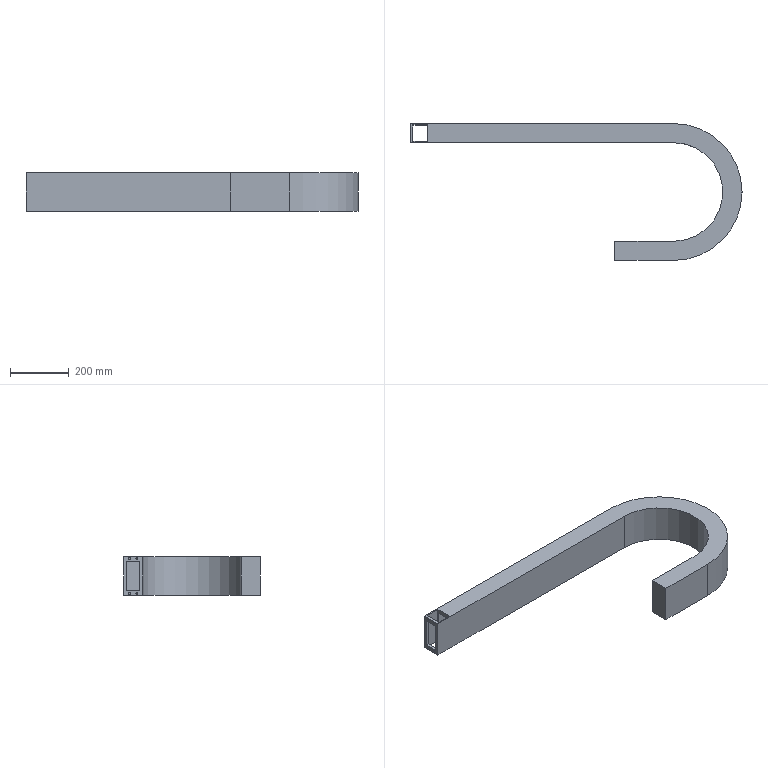Part | SolidWorks | features ICE 3, Extrusion 1 | 1 solid | 31 faces | box 1128 x 465 x 130 mm | volume 13528411 mm3 | plane 21 | cylinder 10 | commonest cylinder face diameters 6 x8 335 x1 465 x1
STEP:
#1=CARTESIAN_POINT('',(-5920.428,254.022,9.));
#2=VERTEX_POINT('',#1);
#3=CARTESIAN_POINT('',(-5920.428,254.022,3.));
#4=VERTEX_POINT('',#3);
#5=CARTESIAN_POINT('',(-5920.428,254.022,6.));
#6=DIRECTION('',(1.,0.,0.));
#7=DIRECTION('',(0.,0.,1.));
#8=AXIS2_PLACEMENT_3D('',#5,#6,#7);
#9=CIRCLE('',#8,3.);
#10=EDGE_CURVE('',#2,#4,#9,.T.);
#11=ORIENTED_EDGE('',*,*,#10,.T.);
#12=CARTESIAN_POINT('',(-5930.428,254.022,3.));
#13=VERTEX_POINT('',#12);
#14=CARTESIAN_POINT('',(-5910.428,254.022,3.));
#15=DIRECTION('',(-1.,0.,0.));
#16=VECTOR('',#15,1000.);
#17=LINE('',#14,#16);
#18=EDGE_CURVE('',#4,#13,#17,.T.);
#19=ORIENTED_EDGE('',*,*,#18,.T.);
#20=CARTESIAN_POINT('',(-5930.428,254.022,9.));
#21=VERTEX_POINT('',#20);
#22=CARTESIAN_POINT('',(-5930.428,254.022,6.));
#23=DIRECTION('',(-1.,0.,0.));
#24=DIRECTION('',(0.,0.,1.));
#25=AXIS2_PLACEMENT_3D('',#22,#23,#24);
#26=CIRCLE('',#25,3.);
#27=EDGE_CURVE('',#13,#21,#26,.T.);
#28=ORIENTED_EDGE('',*,*,#27,.T.);
#29=CARTESIAN_POINT('',(-5910.428,254.022,9.));
#30=DIRECTION('',(-1.,0.,0.));
#31=VECTOR('',#30,1000.);
#32=LINE('',#29,#31);
#33=EDGE_CURVE('',#2,#21,#32,.T.);
#34=ORIENTED_EDGE('',*,*,#33,.F.);
#35=EDGE_LOOP('',(#11,#19,#28,#34));
#36=FACE_OUTER_BOUND('',#35,.T.);
#37=CARTESIAN_POINT('',(-5910.428,254.022,6.));
#38=DIRECTION('',(-1.,0.,0.));
#39=DIRECTION('',(0.,0.,1.));
#40=AXIS2_PLACEMENT_3D('',#37,#38,#39);
#41=CYLINDRICAL_SURFACE('',#40,3.);
#42=ADVANCED_FACE('',(#36),#41,.F.);
#43=CARTESIAN_POINT('',(-5920.428,279.022,127.));
#44=VERTEX_POINT('',#43);
#45=CARTESIAN_POINT('',(-5920.428,279.022,121.));
#46=VERTEX_POINT('',#45);
#47=CARTESIAN_POINT('',(-5920.428,279.022,124.));
#48=DIRECTION('',(1.,0.,0.));
#49=DIRECTION('',(0.,0.,1.));
#50=AXIS2_PLACEMENT_3D('',#47,#48,#49);
#51=CIRCLE('',#50,3.);
#52=EDGE_CURVE('',#44,#46,#51,.T.);
#53=ORIENTED_EDGE('',*,*,#52,.T.);
#54=CARTESIAN_POINT('',(-5930.428,279.022,121.));
#55=VERTEX_POINT('',#54);
#56=CARTESIAN_POINT('',(-5910.428,279.022,121.));
#57=DIRECTION('',(-1.,0.,0.));
#58=VECTOR('',#57,1000.);
#59=LINE('',#56,#58);
#60=EDGE_CURVE('',#46,#55,#59,.T.);
#61=ORIENTED_EDGE('',*,*,#60,.T.);
#62=CARTESIAN_POINT('',(-5930.428,279.022,127.));
#63=VERTEX_POINT('',#62);
#64=CARTESIAN_POINT('',(-5930.428,279.022,124.));
#65=DIRECTION('',(-1.,0.,0.));
#66=DIRECTION('',(0.,0.,1.));
#67=AXIS2_PLACEMENT_3D('',#64,#65,#66);
#68=CIRCLE('',#67,3.);
#69=EDGE_CURVE('',#55,#63,#68,.T.);
#70=ORIENTED_EDGE('',*,*,#69,.T.);
#71=CARTESIAN_POINT('',(-5910.428,279.022,127.));
#72=DIRECTION('',(-1.,0.,0.));
#73=VECTOR('',#72,1000.);
#74=LINE('',#71,#73);
#75=EDGE_CURVE('',#44,#63,#74,.T.);
#76=ORIENTED_EDGE('',*,*,#75,.F.);
#77=EDGE_LOOP('',(#53,#61,#70,#76));
#78=FACE_OUTER_BOUND('',#77,.T.);
#79=CARTESIAN_POINT('',(-5910.428,279.022,124.));
#80=DIRECTION('',(-1.,0.,0.));
#81=DIRECTION('',(0.,0.,1.));
#82=AXIS2_PLACEMENT_3D('',#79,#80,#81);
#83=CYLINDRICAL_SURFACE('',#82,3.);
#84=ADVANCED_FACE('',(#78),#83,.F.);
#85=CARTESIAN_POINT('',(-5920.428,254.022,127.));
#86=VERTEX_POINT('',#85);
#87=CARTESIAN_POINT('',(-5920.428,254.022,121.));
#88=VERTEX_POINT('',#87);
#89=CARTESIAN_POINT('',(-5920.428,254.022,124.));
#90=DIRECTION('',(1.,0.,0.));
#91=DIRECTION('',(0.,0.,1.));
#92=AXIS2_PLACEMENT_3D('',#89,#90,#91);
#93=CIRCLE('',#92,3.);
#94=EDGE_CURVE('',#86,#88,#93,.T.);
#95=ORIENTED_EDGE('',*,*,#94,.T.);
#96=CARTESIAN_POINT('',(-5930.428,254.022,121.));
#97=VERTEX_POINT('',#96);
#98=CARTESIAN_POINT('',(-5910.428,254.022,121.));
#99=DIRECTION('',(-1.,0.,0.));
#100=VECTOR('',#99,1000.);
#101=LINE('',#98,#100);
#102=EDGE_CURVE('',#88,#97,#101,.T.);
#103=ORIENTED_EDGE('',*,*,#102,.T.);
#104=CARTESIAN_POINT('',(-5930.428,254.022,127.));
#105=VERTEX_POINT('',#104);
#106=CARTESIAN_POINT('',(-5930.428,254.022,124.));
#107=DIRECTION('',(-1.,0.,0.));
#108=DIRECTION('',(0.,0.,1.));
#109=AXIS2_PLACEMENT_3D('',#106,#107,#108);
#110=CIRCLE('',#109,3.);
#111=EDGE_CURVE('',#97,#105,#110,.T.);
#112=ORIENTED_EDGE('',*,*,#111,.T.);
#113=CARTESIAN_POINT('',(-5910.428,254.022,127.));
#114=DIRECTION('',(-1.,0.,0.));
#115=VECTOR('',#114,1000.);
#116=LINE('',#113,#115);
#117=EDGE_CURVE('',#86,#105,#116,.T.);
#118=ORIENTED_EDGE('',*,*,#117,.F.);
#119=EDGE_LOOP('',(#95,#103,#112,#118));
#120=FACE_OUTER_BOUND('',#119,.T.);
#121=CARTESIAN_POINT('',(-5910.428,254.022,124.));
#122=DIRECTION('',(-1.,0.,0.));
#123=DIRECTION('',(0.,0.,1.));
#124=AXIS2_PLACEMENT_3D('',#121,#122,#123);
#125=CYLINDRICAL_SURFACE('',#124,3.);
#126=ADVANCED_FACE('',(#120),#125,.F.);
#127=CARTESIAN_POINT('',(-5920.428,279.022,9.));
#128=VERTEX_POINT('',#127);
#129=CARTESIAN_POINT('',(-5920.428,279.022,3.));
#130=VERTEX_POINT('',#129);
#131=CARTESIAN_POINT('',(-5920.428,279.022,6.));
#132=DIRECTION('',(1.,0.,0.));
#133=DIRECTION('',(0.,0.,1.));
#134=AXIS2_PLACEMENT_3D('',#131,#132,#133);
#135=CIRCLE('',#134,3.);
#136=EDGE_CURVE('',#128,#130,#135,.T.);
#137=ORIENTED_EDGE('',*,*,#136,.T.);
#138=CARTESIAN_POINT('',(-5930.428,279.022,3.));
#139=VERTEX_POINT('',#138);
#140=CARTESIAN_POINT('',(-5910.428,279.022,3.));
#141=DIRECTION('',(-1.,0.,0.));
#142=VECTOR('',#141,1000.);
#143=LINE('',#140,#142);
#144=EDGE_CURVE('',#130,#139,#143,.T.);
#145=ORIENTED_EDGE('',*,*,#144,.T.);
#146=CARTESIAN_POINT('',(-5930.428,279.022,9.));
#147=VERTEX_POINT('',#146);
#148=CARTESIAN_POINT('',(-5930.428,279.022,6.));
#149=DIRECTION('',(-1.,0.,0.));
#150=DIRECTION('',(0.,0.,1.));
#151=AXIS2_PLACEMENT_3D('',#148,#149,#150);
#152=CIRCLE('',#151,3.);
#153=EDGE_CURVE('',#139,#147,#152,.T.);
#154=ORIENTED_EDGE('',*,*,#153,.T.);
#155=CARTESIAN_POINT('',(-5910.428,279.022,9.));
#156=DIRECTION('',(-1.,0.,0.));
#157=VECTOR('',#156,1000.);
#158=LINE('',#155,#157);
#159=EDGE_CURVE('',#128,#147,#158,.T.);
#160=ORIENTED_EDGE('',*,*,#159,.F.);
#161=EDGE_LOOP('',(#137,#145,#154,#160));
#162=FACE_OUTER_BOUND('',#161,.T.);
#163=CARTESIAN_POINT('',(-5910.428,279.022,6.));
#164=DIRECTION('',(-1.,0.,0.));
#165=DIRECTION('',(0.,0.,1.));
#166=AXIS2_PLACEMENT_3D('',#163,#164,#165);
#167=CYLINDRICAL_SURFACE('',#166,3.);
#168=ADVANCED_FACE('',(#162),#167,.F.);
#169=CARTESIAN_POINT('',(-5035.428,-165.978,0.));
#170=VERTEX_POINT('',#169);
#171=CARTESIAN_POINT('',(-5035.428,299.022,0.));
#172=VERTEX_POINT('',#171);
#173=CARTESIAN_POINT('',(-5035.428,66.522,0.));
#174=DIRECTION('',(0.,0.,1.));
#175=DIRECTION('',(1.,0.,0.));
#176=AXIS2_PLACEMENT_3D('',#173,#174,#175);
#177=CIRCLE('',#176,232.5);
#178=EDGE_CURVE('',#170,#172,#177,.T.);
#179=ORIENTED_EDGE('',*,*,#178,.T.);
#180=CARTESIAN_POINT('',(-5035.428,299.022,130.));
#181=VERTEX_POINT('',#180);
#182=CARTESIAN_POINT('',(-5035.428,299.022,130.));
#183=DIRECTION('',(0.,0.,-1.));
#184=VECTOR('',#183,1000.);
#185=LINE('',#182,#184);
#186=EDGE_CURVE('',#181,#172,#185,.T.);
#187=ORIENTED_EDGE('',*,*,#186,.F.);
#188=CARTESIAN_POINT('',(-5035.428,-165.978,130.));
#189=VERTEX_POINT('',#188);
#190=CARTESIAN_POINT('',(-5035.428,66.522,130.));
#191=DIRECTION('',(0.,0.,1.));
#192=DIRECTION('',(1.,0.,0.));
#193=AXIS2_PLACEMENT_3D('',#190,#191,#192);
#194=CIRCLE('',#193,232.5);
#195=EDGE_CURVE('',#189,#181,#194,.T.);
#196=ORIENTED_EDGE('',*,*,#195,.F.);
#197=CARTESIAN_POINT('',(-5035.428,-165.978,130.));
#198=DIRECTION('',(0.,0.,-1.));
#199=VECTOR('',#198,1000.);
#200=LINE('',#197,#199);
#201=EDGE_CURVE('',#189,#170,#200,.T.);
#202=ORIENTED_EDGE('',*,*,#201,.T.);
#203=EDGE_LOOP('',(#179,#187,#196,#202));
#204=FACE_OUTER_BOUND('',#203,.T.);
#205=CARTESIAN_POINT('',(-5035.428,66.522,130.));
#206=DIRECTION('',(0.,0.,-1.));
#207=DIRECTION('',(-1.,0.,0.));
#208=AXIS2_PLACEMENT_3D('',#205,#206,#207);
#209=CYLINDRICAL_SURFACE('',#208,232.5);
#210=ADVANCED_FACE('',(#204),#209,.T.);
#211=CARTESIAN_POINT('',(-5930.428,299.022,0.));
#212=VERTEX_POINT('',#211);
#213=CARTESIAN_POINT('',(-5035.428,299.022,0.));
#214=DIRECTION('',(-1.,0.,0.));
#215=VECTOR('',#214,1000.);
#216=LINE('',#213,#215);
#217=EDGE_CURVE('',#172,#212,#216,.T.);
#218=ORIENTED_EDGE('',*,*,#217,.T.);
#219=CARTESIAN_POINT('',(-5930.428,299.022,130.));
#220=VERTEX_POINT('',#219);
#221=CARTESIAN_POINT('',(-5930.428,299.022,130.));
#222=DIRECTION('',(0.,0.,-1.));
#223=VECTOR('',#222,1000.);
#224=LINE('',#221,#223);
#225=EDGE_CURVE('',#220,#212,#224,.T.);
#226=ORIENTED_EDGE('',*,*,#225,.F.);
#227=CARTESIAN_POINT('',(-5035.428,299.022,130.));
#228=DIRECTION('',(-1.,0.,0.));
#229=VECTOR('',#228,1000.);
#230=LINE('',#227,#229);
#231=EDGE_CURVE('',#181,#220,#230,.T.);
#232=ORIENTED_EDGE('',*,*,#231,.F.);
#233=ORIENTED_EDGE('',*,*,#186,.T.);
#234=EDGE_LOOP('',(#218,#226,#232,#233));
#235=FACE_OUTER_BOUND('',#234,.T.);
#236=CARTESIAN_POINT('',(-5035.428,299.022,130.));
#237=DIRECTION('',(0.,-1.,0.));
#238=DIRECTION('',(1.,0.,0.));
#239=AXIS2_PLACEMENT_3D('',#236,#237,#238);
#240=PLANE('',#239);
#241=ADVANCED_FACE('',(#235),#240,.F.);
#242=CARTESIAN_POINT('',(-5930.428,244.022,15.));
#243=VERTEX_POINT('',#242);
#244=CARTESIAN_POINT('',(-5930.428,244.022,115.));
#245=VERTEX_POINT('',#244);
#246=CARTESIAN_POINT('',(-5930.428,244.022,15.));
#247=DIRECTION('',(0.,0.,1.));
#248=VECTOR('',#247,1000.);
#249=LINE('',#246,#248);
#250=EDGE_CURVE('',#243,#245,#249,.T.);
#251=ORIENTED_EDGE('',*,*,#250,.F.);
#252=CARTESIAN_POINT('',(-5930.428,289.022,15.));
#253=VERTEX_POINT('',#252);
#254=CARTESIAN_POINT('',(-5930.428,289.022,15.));
#255=DIRECTION('',(0.,-1.,0.));
#256=VECTOR('',#255,1000.);
#257=LINE('',#254,#256);
#258=EDGE_CURVE('',#253,#243,#257,.T.);
#259=ORIENTED_EDGE('',*,*,#258,.F.);
#260=CARTESIAN_POINT('',(-5930.428,289.022,115.));
#261=VERTEX_POINT('',#260);
#262=CARTESIAN_POINT('',(-5930.428,289.022,15.));
#263=DIRECTION('',(0.,0.,-1.));
#264=VECTOR('',#263,1000.);
#265=LINE('',#262,#264);
#266=EDGE_CURVE('',#261,#253,#265,.T.);
#267=ORIENTED_EDGE('',*,*,#266,.F.);
#268=CARTESIAN_POINT('',(-5930.428,289.022,115.));
#269=DIRECTION('',(0.,1.,0.));
#270=VECTOR('',#269,1000.);
#271=LINE('',#268,#270);
#272=EDGE_CURVE('',#245,#261,#271,.T.);
#273=ORIENTED_EDGE('',*,*,#272,.F.);
#274=EDGE_LOOP('',(#251,#259,#267,#273));
#275=FACE_BOUND('',#274,.T.);
#276=CARTESIAN_POINT('',(-5930.428,254.022,6.));
#277=DIRECTION('',(-1.,0.,0.));
#278=DIRECTION('',(0.,0.,1.));
#279=AXIS2_PLACEMENT_3D('',#276,#277,#278);
#280=CIRCLE('',#279,3.);
#281=EDGE_CURVE('',#21,#13,#280,.T.);
#282=ORIENTED_EDGE('',*,*,#281,.F.);
#283=ORIENTED_EDGE('',*,*,#27,.F.);
#284=EDGE_LOOP('',(#282,#283));
#285=FACE_BOUND('',#284,.T.);
#286=CARTESIAN_POINT('',(-5930.428,279.022,124.));
#287=DIRECTION('',(-1.,0.,0.));
#288=DIRECTION('',(0.,0.,1.));
#289=AXIS2_PLACEMENT_3D('',#286,#287,#288);
#290=CIRCLE('',#289,3.);
#291=EDGE_CURVE('',#63,#55,#290,.T.);
#292=ORIENTED_EDGE('',*,*,#291,.F.);
#293=ORIENTED_EDGE('',*,*,#69,.F.);
#294=EDGE_LOOP('',(#292,#293));
#295=FACE_BOUND('',#294,.T.);
#296=CARTESIAN_POINT('',(-5930.428,254.022,124.));
#297=DIRECTION('',(-1.,0.,0.));
#298=DIRECTION('',(0.,0.,1.));
#299=AXIS2_PLACEMENT_3D('',#296,#297,#298);
#300=CIRCLE('',#299,3.);
#301=EDGE_CURVE('',#105,#97,#300,.T.);
#302=ORIENTED_EDGE('',*,*,#301,.F.);
#303=ORIENTED_EDGE('',*,*,#111,.F.);
#304=EDGE_LOOP('',(#302,#303));
#305=FACE_BOUND('',#304,.T.);
#306=CARTESIAN_POINT('',(-5930.428,279.022,6.));
#307=DIRECTION('',(-1.,0.,0.));
#308=DIRECTION('',(0.,0.,1.));
#309=AXIS2_PLACEMENT_3D('',#306,#307,#308);
#310=CIRCLE('',#309,3.);
#311=EDGE_CURVE('',#147,#139,#310,.T.);
#312=ORIENTED_EDGE('',*,*,#311,.F.);
#313=ORIENTED_EDGE('',*,*,#153,.F.);
#314=EDGE_LOOP('',(#312,#313));
#315=FACE_BOUND('',#314,.T.);
#316=CARTESIAN_POINT('',(-5930.428,234.022,0.));
#317=VERTEX_POINT('',#316);
#318=CARTESIAN_POINT('',(-5930.428,299.022,0.));
#319=DIRECTION('',(0.,-1.,0.));
#320=VECTOR('',#319,1000.);
#321=LINE('',#318,#320);
#322=EDGE_CURVE('',#212,#317,#321,.T.);
#323=ORIENTED_EDGE('',*,*,#322,.T.);
#324=CARTESIAN_POINT('',(-5930.428,234.022,130.));
#325=VERTEX_POINT('',#324);
#326=CARTESIAN_POINT('',(-5930.428,234.022,130.));
#327=DIRECTION('',(0.,0.,-1.));
#328=VECTOR('',#327,1000.);
#329=LINE('',#326,#328);
#330=EDGE_CURVE('',#325,#317,#329,.T.);
#331=ORIENTED_EDGE('',*,*,#330,.F.);
#332=CARTESIAN_POINT('',(-5930.428,299.022,130.));
#333=DIRECTION('',(0.,-1.,0.));
#334=VECTOR('',#333,1000.);
#335=LINE('',#332,#334);
#336=EDGE_CURVE('',#220,#325,#335,.T.);
#337=ORIENTED_EDGE('',*,*,#336,.F.);
#338=ORIENTED_EDGE('',*,*,#225,.T.);
#339=EDGE_LOOP('',(#323,#331,#337,#338));
#340=FACE_OUTER_BOUND('',#339,.T.);
#341=CARTESIAN_POINT('',(-5930.428,299.022,130.));
#342=DIRECTION('',(1.,0.,0.));
#343=DIRECTION('',(0.,0.,-1.));
#344=AXIS2_PLACEMENT_3D('',#341,#342,#343);
#345=PLANE('',#344);
#346=ADVANCED_FACE('',(#275,#285,#295,#305,#315,#340),#345,.F.);
#347=CARTESIAN_POINT('',(-5035.428,234.022,0.));
#348=VERTEX_POINT('',#347);
#349=CARTESIAN_POINT('',(-5035.428,234.022,0.));
#350=DIRECTION('',(1.,0.,0.));
#351=VECTOR('',#350,1000.);
#352=LINE('',#349,#351);
#353=EDGE_CURVE('',#317,#348,#352,.T.);
#354=ORIENTED_EDGE('',*,*,#353,.T.);
#355=CARTESIAN_POINT('',(-5035.428,234.022,130.));
#356=VERTEX_POINT('',#355);
#357=CARTESIAN_POINT('',(-5035.428,234.022,130.));
#358=DIRECTION('',(0.,0.,-1.));
#359=VECTOR('',#358,1000.);
#360=LINE('',#357,#359);
#361=EDGE_CURVE('',#356,#348,#360,.T.);
#362=ORIENTED_EDGE('',*,*,#361,.F.);
#363=CARTESIAN_POINT('',(-5035.428,234.022,130.));
#364=DIRECTION('',(1.,0.,0.));
#365=VECTOR('',#364,1000.);
#366=LINE('',#363,#365);
#367=EDGE_CURVE('',#325,#356,#366,.T.);
#368=ORIENTED_EDGE('',*,*,#367,.F.);
#369=ORIENTED_EDGE('',*,*,#330,.T.);
#370=EDGE_LOOP('',(#354,#362,#368,#369));
#371=FACE_OUTER_BOUND('',#370,.T.);
#372=CARTESIAN_POINT('',(-5035.428,234.022,130.));
#373=DIRECTION('',(0.,1.,0.));
#374=DIRECTION('',(-1.,0.,0.));
#375=AXIS2_PLACEMENT_3D('',#372,#373,#374);
#376=PLANE('',#375);
#377=ADVANCED_FACE('',(#371),#376,.F.);
#378=CARTESIAN_POINT('',(-5035.428,-100.978,0.));
#379=VERTEX_POINT('',#378);
#380=CARTESIAN_POINT('',(-5035.428,66.522,0.));
#381=DIRECTION('',(0.,0.,-1.));
#382=DIRECTION('',(1.,0.,0.));
#383=AXIS2_PLACEMENT_3D('',#380,#381,#382);
#384=CIRCLE('',#383,167.5);
#385=EDGE_CURVE('',#348,#379,#384,.T.);
#386=ORIENTED_EDGE('',*,*,#385,.T.);
#387=CARTESIAN_POINT('',(-5035.428,-100.978,130.));
#388=VERTEX_POINT('',#387);
#389=CARTESIAN_POINT('',(-5035.428,-100.978,130.));
#390=DIRECTION('',(0.,0.,-1.));
#391=VECTOR('',#390,1000.);
#392=LINE('',#389,#391);
#393=EDGE_CURVE('',#388,#379,#392,.T.);
#394=ORIENTED_EDGE('',*,*,#393,.F.);
#395=CARTESIAN_POINT('',(-5035.428,66.522,130.));
#396=DIRECTION('',(0.,0.,-1.));
#397=DIRECTION('',(1.,0.,0.));
#398=AXIS2_PLACEMENT_3D('',#395,#396,#397);
#399=CIRCLE('',#398,167.5);
#400=EDGE_CURVE('',#356,#388,#399,.T.);
#401=ORIENTED_EDGE('',*,*,#400,.F.);
#402=ORIENTED_EDGE('',*,*,#361,.T.);
#403=EDGE_LOOP('',(#386,#394,#401,#402));
#404=FACE_OUTER_BOUND('',#403,.T.);
#405=CARTESIAN_POINT('',(-5035.428,66.522,130.));
#406=DIRECTION('',(0.,0.,-1.));
#407=DIRECTION('',(-1.,0.,0.));
#408=AXIS2_PLACEMENT_3D('',#405,#406,#407);
#409=CYLINDRICAL_SURFACE('',#408,167.5);
#410=ADVANCED_FACE('',(#404),#409,.F.);
#411=CARTESIAN_POINT('',(-5235.428,-100.978,0.));
#412=VERTEX_POINT('',#411);
#413=CARTESIAN_POINT('',(-5035.428,-100.978,0.));
#414=DIRECTION('',(-1.,0.,0.));
#415=VECTOR('',#414,1000.);
#416=LINE('',#413,#415);
#417=EDGE_CURVE('',#379,#412,#416,.T.);
#418=ORIENTED_EDGE('',*,*,#417,.T.);
#419=CARTESIAN_POINT('',(-5235.428,-100.978,130.));
#420=VERTEX_POINT('',#419);
#421=CARTESIAN_POINT('',(-5235.428,-100.978,130.));
#422=DIRECTION('',(0.,0.,-1.));
#423=VECTOR('',#422,1000.);
#424=LINE('',#421,#423);
#425=EDGE_CURVE('',#420,#412,#424,.T.);
#426=ORIENTED_EDGE('',*,*,#425,.F.);
#427=CARTESIAN_POINT('',(-5035.428,-100.978,130.));
#428=DIRECTION('',(-1.,0.,0.));
#429=VECTOR('',#428,1000.);
#430=LINE('',#427,#429);
#431=EDGE_CURVE('',#388,#420,#430,.T.);
#432=ORIENTED_EDGE('',*,*,#431,.F.);
#433=ORIENTED_EDGE('',*,*,#393,.T.);
#434=EDGE_LOOP('',(#418,#426,#432,#433));
#435=FACE_OUTER_BOUND('',#434,.T.);
#436=CARTESIAN_POINT('',(-5035.428,-100.978,130.));
#437=DIRECTION('',(0.,-1.,0.));
#438=DIRECTION('',(1.,0.,0.));
#439=AXIS2_PLACEMENT_3D('',#436,#437,#438);
#440=PLANE('',#439);
#441=ADVANCED_FACE('',(#435),#440,.F.);
#442=CARTESIAN_POINT('',(-5235.428,-165.978,0.));
#443=VERTEX_POINT('',#442);
#444=CARTESIAN_POINT('',(-5235.428,-165.978,0.));
#445=DIRECTION('',(0.,-1.,0.));
#446=VECTOR('',#445,1000.);
#447=LINE('',#444,#446);
#448=EDGE_CURVE('',#412,#443,#447,.T.);
#449=ORIENTED_EDGE('',*,*,#448,.T.);
#450=CARTESIAN_POINT('',(-5235.428,-165.978,130.));
#451=VERTEX_POINT('',#450);
#452=CARTESIAN_POINT('',(-5235.428,-165.978,130.));
#453=DIRECTION('',(0.,0.,-1.));
#454=VECTOR('',#453,1000.);
#455=LINE('',#452,#454);
#456=EDGE_CURVE('',#451,#443,#455,.T.);
#457=ORIENTED_EDGE('',*,*,#456,.F.);
#458=CARTESIAN_POINT('',(-5235.428,-165.978,130.));
#459=DIRECTION('',(0.,-1.,0.));
#460=VECTOR('',#459,1000.);
#461=LINE('',#458,#460);
#462=EDGE_CURVE('',#420,#451,#461,.T.);
#463=ORIENTED_EDGE('',*,*,#462,.F.);
#464=ORIENTED_EDGE('',*,*,#425,.T.);
#465=EDGE_LOOP('',(#449,#457,#463,#464));
#466=FACE_OUTER_BOUND('',#465,.T.);
#467=CARTESIAN_POINT('',(-5235.428,-165.978,130.));
#468=DIRECTION('',(1.,0.,0.));
#469=DIRECTION('',(0.,0.,-1.));
#470=AXIS2_PLACEMENT_3D('',#467,#468,#469);
#471=PLANE('',#470);
#472=ADVANCED_FACE('',(#466),#471,.F.);
#473=CARTESIAN_POINT('',(-5035.428,-165.978,0.));
#474=DIRECTION('',(1.,0.,0.));
#475=VECTOR('',#474,1000.);
#476=LINE('',#473,#475);
#477=EDGE_CURVE('',#443,#170,#476,.T.);
#478=ORIENTED_EDGE('',*,*,#477,.T.);
#479=ORIENTED_EDGE('',*,*,#201,.F.);
#480=CARTESIAN_POINT('',(-5035.428,-165.978,130.));
#481=DIRECTION('',(1.,0.,0.));
#482=VECTOR('',#481,1000.);
#483=LINE('',#480,#482);
#484=EDGE_CURVE('',#451,#189,#483,.T.);
#485=ORIENTED_EDGE('',*,*,#484,.F.);
#486=ORIENTED_EDGE('',*,*,#456,.T.);
#487=EDGE_LOOP('',(#478,#479,#485,#486));
#488=FACE_OUTER_BOUND('',#487,.T.);
#489=CARTESIAN_POINT('',(-5035.428,-165.978,130.));
#490=DIRECTION('',(0.,1.,0.));
#491=DIRECTION('',(-1.,0.,0.));
#492=AXIS2_PLACEMENT_3D('',#489,#490,#491);
#493=PLANE('',#492);
#494=ADVANCED_FACE('',(#488),#493,.F.);
#495=CARTESIAN_POINT('',(-5920.428,294.022,130.));
#496=VERTEX_POINT('',#495);
#497=CARTESIAN_POINT('',(-5920.428,239.022,130.));
#498=VERTEX_POINT('',#497);
#499=CARTESIAN_POINT('',(-5920.428,294.022,130.));
#500=DIRECTION('',(0.,-1.,0.));
#501=VECTOR('',#500,1000.);
#502=LINE('',#499,#501);
#503=EDGE_CURVE('',#496,#498,#502,.T.);
#504=ORIENTED_EDGE('',*,*,#503,.F.);
#505=CARTESIAN_POINT('',(-5870.428,294.022,130.));
#506=VERTEX_POINT('',#505);
#507=CARTESIAN_POINT('',(-5920.428,294.022,130.));
#508=DIRECTION('',(-1.,0.,0.));
#509=VECTOR('',#508,1000.);
#510=LINE('',#507,#509);
#511=EDGE_CURVE('',#506,#496,#510,.T.);
#512=ORIENTED_EDGE('',*,*,#511,.F.);
#513=CARTESIAN_POINT('',(-5870.428,239.022,130.));
#514=VERTEX_POINT('',#513);
#515=CARTESIAN_POINT('',(-5870.428,294.022,130.));
#516=DIRECTION('',(0.,1.,0.));
#517=VECTOR('',#516,1000.);
#518=LINE('',#515,#517);
#519=EDGE_CURVE('',#514,#506,#518,.T.);
#520=ORIENTED_EDGE('',*,*,#519,.F.);
#521=CARTESIAN_POINT('',(-5920.428,239.022,130.));
#522=DIRECTION('',(1.,0.,0.));
#523=VECTOR('',#522,1000.);
#524=LINE('',#521,#523);
#525=EDGE_CURVE('',#498,#514,#524,.T.);
#526=ORIENTED_EDGE('',*,*,#525,.F.);
#527=EDGE_LOOP('',(#504,#512,#520,#526));
#528=FACE_BOUND('',#527,.T.);
#529=ORIENTED_EDGE('',*,*,#195,.T.);
#530=ORIENTED_EDGE('',*,*,#231,.T.);
#531=ORIENTED_EDGE('',*,*,#336,.T.);
#532=ORIENTED_EDGE('',*,*,#367,.T.);
#533=ORIENTED_EDGE('',*,*,#400,.T.);
#534=ORIENTED_EDGE('',*,*,#431,.T.);
#535=ORIENTED_EDGE('',*,*,#462,.T.);
#536=ORIENTED_EDGE('',*,*,#484,.T.);
#537=EDGE_LOOP('',(#529,#530,#531,#532,#533,#534,#535,#536));
#538=FACE_OUTER_BOUND('',#537,.T.);
#539=CARTESIAN_POINT('',(-5035.428,66.522,130.));
#540=DIRECTION('',(0.,0.,1.));
#541=DIRECTION('',(1.,0.,0.));
#542=AXIS2_PLACEMENT_3D('',#539,#540,#541);
#543=PLANE('',#542);
#544=ADVANCED_FACE('',(#528,#538),#543,.T.);
#545=CARTESIAN_POINT('',(-5870.428,294.022,0.));
#546=VERTEX_POINT('',#545);
#547=CARTESIAN_POINT('',(-5920.428,294.022,0.));
#548=VERTEX_POINT('',#547);
#549=CARTESIAN_POINT('',(-5035.428,294.022,0.));
#550=DIRECTION('',(-1.,0.,0.));
#551=VECTOR('',#550,1000.);
#552=LINE('',#549,#551);
#553=EDGE_CURVE('',#546,#548,#552,.T.);
#554=ORIENTED_EDGE('',*,*,#553,.T.);
#555=CARTESIAN_POINT('',(-5920.428,239.022,0.));
#556=VERTEX_POINT('',#555);
#557=CARTESIAN_POINT('',(-5920.428,66.522,0.));
#558=DIRECTION('',(0.,-1.,0.));
#559=VECTOR('',#558,1000.);
#560=LINE('',#557,#559);
#561=EDGE_CURVE('',#548,#556,#560,.T.);
#562=ORIENTED_EDGE('',*,*,#561,.T.);
#563=CARTESIAN_POINT('',(-5870.428,239.022,0.));
#564=VERTEX_POINT('',#563);
#565=CARTESIAN_POINT('',(-5035.428,239.022,0.));
#566=DIRECTION('',(1.,0.,0.));
#567=VECTOR('',#566,1000.);
#568=LINE('',#565,#567);
#569=EDGE_CURVE('',#556,#564,#568,.T.);
#570=ORIENTED_EDGE('',*,*,#569,.T.);
#571=CARTESIAN_POINT('',(-5870.428,66.522,0.));
#572=DIRECTION('',(0.,1.,0.));
#573=VECTOR('',#572,1000.);
#574=LINE('',#571,#573);
#575=EDGE_CURVE('',#564,#546,#574,.T.);
#576=ORIENTED_EDGE('',*,*,#575,.T.);
#577=EDGE_LOOP('',(#554,#562,#570,#576));
#578=FACE_BOUND('',#577,.T.);
#579=ORIENTED_EDGE('',*,*,#178,.F.);
#580=ORIENTED_EDGE('',*,*,#477,.F.);
#581=ORIENTED_EDGE('',*,*,#448,.F.);
#582=ORIENTED_EDGE('',*,*,#417,.F.);
#583=ORIENTED_EDGE('',*,*,#385,.F.);
#584=ORIENTED_EDGE('',*,*,#353,.F.);
#585=ORIENTED_EDGE('',*,*,#322,.F.);
#586=ORIENTED_EDGE('',*,*,#217,.F.);
#587=EDGE_LOOP('',(#579,#580,#581,#582,#583,#584,#585,#586));
#588=FACE_OUTER_BOUND('',#587,.T.);
#589=CARTESIAN_POINT('',(-5035.428,66.522,0.));
#590=DIRECTION('',(0.,0.,1.));
#591=DIRECTION('',(1.,0.,0.));
#592=AXIS2_PLACEMENT_3D('',#589,#590,#591);
#593=PLANE('',#592);
#594=ADVANCED_FACE('',(#578,#588),#593,.F.);
#595=ORIENTED_EDGE('',*,*,#144,.F.);
#596=CARTESIAN_POINT('',(-5920.428,279.022,6.));
#597=DIRECTION('',(1.,0.,0.));
#598=DIRECTION('',(0.,0.,1.));
#599=AXIS2_PLACEMENT_3D('',#596,#597,#598);
#600=CIRCLE('',#599,3.);
#601=EDGE_CURVE('',#130,#128,#600,.T.);
#602=ORIENTED_EDGE('',*,*,#601,.T.);
#603=ORIENTED_EDGE('',*,*,#159,.T.);
#604=ORIENTED_EDGE('',*,*,#311,.T.);
#605=EDGE_LOOP('',(#595,#602,#603,#604));
#606=FACE_OUTER_BOUND('',#605,.T.);
#607=CARTESIAN_POINT('',(-5910.428,279.022,6.));
#608=DIRECTION('',(-1.,0.,0.));
#609=DIRECTION('',(0.,0.,1.));
#610=AXIS2_PLACEMENT_3D('',#607,#608,#609);
#611=CYLINDRICAL_SURFACE('',#610,3.);
#612=ADVANCED_FACE('',(#606),#611,.F.);
#613=ORIENTED_EDGE('',*,*,#102,.F.);
#614=CARTESIAN_POINT('',(-5920.428,254.022,124.));
#615=DIRECTION('',(1.,0.,0.));
#616=DIRECTION('',(0.,0.,1.));
#617=AXIS2_PLACEMENT_3D('',#614,#615,#616);
#618=CIRCLE('',#617,3.);
#619=EDGE_CURVE('',#88,#86,#618,.T.);
#620=ORIENTED_EDGE('',*,*,#619,.T.);
#621=ORIENTED_EDGE('',*,*,#117,.T.);
#622=ORIENTED_EDGE('',*,*,#301,.T.);
#623=EDGE_LOOP('',(#613,#620,#621,#622));
#624=FACE_OUTER_BOUND('',#623,.T.);
#625=CARTESIAN_POINT('',(-5910.428,254.022,124.));
#626=DIRECTION('',(-1.,0.,0.));
#627=DIRECTION('',(0.,0.,1.));
#628=AXIS2_PLACEMENT_3D('',#625,#626,#627);
#629=CYLINDRICAL_SURFACE('',#628,3.);
#630=ADVANCED_FACE('',(#624),#629,.F.);
#631=ORIENTED_EDGE('',*,*,#60,.F.);
#632=CARTESIAN_POINT('',(-5920.428,279.022,124.));
#633=DIRECTION('',(1.,0.,0.));
#634=DIRECTION('',(0.,0.,1.));
#635=AXIS2_PLACEMENT_3D('',#632,#633,#634);
#636=CIRCLE('',#635,3.);
#637=EDGE_CURVE('',#46,#44,#636,.T.);
#638=ORIENTED_EDGE('',*,*,#637,.T.);
#639=ORIENTED_EDGE('',*,*,#75,.T.);
#640=ORIENTED_EDGE('',*,*,#291,.T.);
#641=EDGE_LOOP('',(#631,#638,#639,#640));
#642=FACE_OUTER_BOUND('',#641,.T.);
#643=CARTESIAN_POINT('',(-5910.428,279.022,124.));
#644=DIRECTION('',(-1.,0.,0.));
#645=DIRECTION('',(0.,0.,1.));
#646=AXIS2_PLACEMENT_3D('',#643,#644,#645);
#647=CYLINDRICAL_SURFACE('',#646,3.);
#648=ADVANCED_FACE('',(#642),#647,.F.);
#649=ORIENTED_EDGE('',*,*,#18,.F.);
#650=CARTESIAN_POINT('',(-5920.428,254.022,6.));
#651=DIRECTION('',(1.,0.,0.));
#652=DIRECTION('',(0.,0.,1.));
#653=AXIS2_PLACEMENT_3D('',#650,#651,#652);
#654=CIRCLE('',#653,3.);
#655=EDGE_CURVE('',#4,#2,#654,.T.);
#656=ORIENTED_EDGE('',*,*,#655,.T.);
#657=ORIENTED_EDGE('',*,*,#33,.T.);
#658=ORIENTED_EDGE('',*,*,#281,.T.);
#659=EDGE_LOOP('',(#649,#656,#657,#658));
#660=FACE_OUTER_BOUND('',#659,.T.);
#661=CARTESIAN_POINT('',(-5910.428,254.022,6.));
#662=DIRECTION('',(-1.,0.,0.));
#663=DIRECTION('',(0.,0.,1.));
#664=AXIS2_PLACEMENT_3D('',#661,#662,#663);
#665=CYLINDRICAL_SURFACE('',#664,3.);
#666=ADVANCED_FACE('',(#660),#665,.F.);
#667=CARTESIAN_POINT('',(-5870.428,294.022,-20.));
#668=DIRECTION('',(0.,0.,1.));
#669=VECTOR('',#668,1000.);
#670=LINE('',#667,#669);
#671=EDGE_CURVE('',#546,#506,#670,.T.);
#672=ORIENTED_EDGE('',*,*,#671,.T.);
#673=ORIENTED_EDGE('',*,*,#511,.T.);
#674=CARTESIAN_POINT('',(-5920.428,294.022,-20.));
#675=DIRECTION('',(0.,0.,1.));
#676=VECTOR('',#675,1000.);
#677=LINE('',#674,#676);
#678=EDGE_CURVE('',#548,#496,#677,.T.);
#679=ORIENTED_EDGE('',*,*,#678,.F.);
#680=ORIENTED_EDGE('',*,*,#553,.F.);
#681=EDGE_LOOP('',(#672,#673,#679,#680));
#682=FACE_OUTER_BOUND('',#681,.T.);
#683=CARTESIAN_POINT('',(-5920.428,294.022,-20.));
#684=DIRECTION('',(0.,1.,0.));
#685=DIRECTION('',(0.,0.,1.));
#686=AXIS2_PLACEMENT_3D('',#683,#684,#685);
#687=PLANE('',#686);
#688=ADVANCED_FACE('',(#682),#687,.F.);
#689=CARTESIAN_POINT('',(-5870.428,244.022,115.));
#690=VERTEX_POINT('',#689);
#691=CARTESIAN_POINT('',(-5870.428,244.022,15.));
#692=VERTEX_POINT('',#691);
#693=CARTESIAN_POINT('',(-5870.428,244.022,-20.));
#694=DIRECTION('',(0.,0.,-1.));
#695=VECTOR('',#694,1000.);
#696=LINE('',#693,#695);
#697=EDGE_CURVE('',#690,#692,#696,.T.);
#698=ORIENTED_EDGE('',*,*,#697,.T.);
#699=CARTESIAN_POINT('',(-5870.428,289.022,15.));
#700=VERTEX_POINT('',#699);
#701=CARTESIAN_POINT('',(-5870.428,294.022,15.));
#702=DIRECTION('',(0.,1.,0.));
#703=VECTOR('',#702,1000.);
#704=LINE('',#701,#703);
#705=EDGE_CURVE('',#692,#700,#704,.T.);
#706=ORIENTED_EDGE('',*,*,#705,.T.);
#707=CARTESIAN_POINT('',(-5870.428,289.022,115.));
#708=VERTEX_POINT('',#707);
#709=CARTESIAN_POINT('',(-5870.428,289.022,-20.));
#710=DIRECTION('',(0.,0.,1.));
#711=VECTOR('',#710,1000.);
#712=LINE('',#709,#711);
#713=EDGE_CURVE('',#700,#708,#712,.T.);
#714=ORIENTED_EDGE('',*,*,#713,.T.);
#715=CARTESIAN_POINT('',(-5870.428,294.022,115.));
#716=DIRECTION('',(0.,-1.,0.));
#717=VECTOR('',#716,1000.);
#718=LINE('',#715,#717);
#719=EDGE_CURVE('',#708,#690,#718,.T.);
#720=ORIENTED_EDGE('',*,*,#719,.T.);
#721=EDGE_LOOP('',(#698,#706,#714,#720));
#722=FACE_BOUND('',#721,.T.);
#723=CARTESIAN_POINT('',(-5870.428,239.022,-20.));
#724=DIRECTION('',(0.,0.,1.));
#725=VECTOR('',#724,1000.);
#726=LINE('',#723,#725);
#727=EDGE_CURVE('',#564,#514,#726,.T.);
#728=ORIENTED_EDGE('',*,*,#727,.T.);
#729=ORIENTED_EDGE('',*,*,#519,.T.);
#730=ORIENTED_EDGE('',*,*,#671,.F.);
#731=ORIENTED_EDGE('',*,*,#575,.F.);
#732=EDGE_LOOP('',(#728,#729,#730,#731));
#733=FACE_OUTER_BOUND('',#732,.T.);
#734=CARTESIAN_POINT('',(-5870.428,294.022,-20.));
#735=DIRECTION('',(1.,0.,0.));
#736=DIRECTION('',(0.,0.,-1.));
#737=AXIS2_PLACEMENT_3D('',#734,#735,#736);
#738=PLANE('',#737);
#739=ADVANCED_FACE('',(#722,#733),#738,.F.);
#740=CARTESIAN_POINT('',(-5920.428,239.022,-20.));
#741=DIRECTION('',(0.,0.,1.));
#742=VECTOR('',#741,1000.);
#743=LINE('',#740,#742);
#744=EDGE_CURVE('',#556,#498,#743,.T.);
#745=ORIENTED_EDGE('',*,*,#744,.T.);
#746=ORIENTED_EDGE('',*,*,#525,.T.);
#747=ORIENTED_EDGE('',*,*,#727,.F.);
#748=ORIENTED_EDGE('',*,*,#569,.F.);
#749=EDGE_LOOP('',(#745,#746,#747,#748));
#750=FACE_OUTER_BOUND('',#749,.T.);
#751=CARTESIAN_POINT('',(-5920.428,239.022,-20.));
#752=DIRECTION('',(0.,-1.,0.));
#753=DIRECTION('',(0.,0.,-1.));
#754=AXIS2_PLACEMENT_3D('',#751,#752,#753);
#755=PLANE('',#754);
#756=ADVANCED_FACE('',(#750),#755,.F.);
#757=CARTESIAN_POINT('',(-5920.428,289.022,115.));
#758=VERTEX_POINT('',#757);
#759=CARTESIAN_POINT('',(-5920.428,289.022,15.));
#760=VERTEX_POINT('',#759);
#761=CARTESIAN_POINT('',(-5920.428,289.022,-20.));
#762=DIRECTION('',(0.,0.,-1.));
#763=VECTOR('',#762,1000.);
#764=LINE('',#761,#763);
#765=EDGE_CURVE('',#758,#760,#764,.T.);
#766=ORIENTED_EDGE('',*,*,#765,.T.);
#767=CARTESIAN_POINT('',(-5920.428,244.022,15.));
#768=VERTEX_POINT('',#767);
#769=CARTESIAN_POINT('',(-5920.428,294.022,15.));
#770=DIRECTION('',(0.,-1.,0.));
#771=VECTOR('',#770,1000.);
#772=LINE('',#769,#771);
#773=EDGE_CURVE('',#760,#768,#772,.T.);
#774=ORIENTED_EDGE('',*,*,#773,.T.);
#775=CARTESIAN_POINT('',(-5920.428,244.022,115.));
#776=VERTEX_POINT('',#775);
#777=CARTESIAN_POINT('',(-5920.428,244.022,-20.));
#778=DIRECTION('',(0.,0.,1.));
#779=VECTOR('',#778,1000.);
#780=LINE('',#777,#779);
#781=EDGE_CURVE('',#768,#776,#780,.T.);
#782=ORIENTED_EDGE('',*,*,#781,.T.);
#783=CARTESIAN_POINT('',(-5920.428,294.022,115.));
#784=DIRECTION('',(0.,1.,0.));
#785=VECTOR('',#784,1000.);
#786=LINE('',#783,#785);
#787=EDGE_CURVE('',#776,#758,#786,.T.);
#788=ORIENTED_EDGE('',*,*,#787,.T.);
#789=EDGE_LOOP('',(#766,#774,#782,#788));
#790=FACE_BOUND('',#789,.T.);
#791=ORIENTED_EDGE('',*,*,#94,.F.);
#792=ORIENTED_EDGE('',*,*,#619,.F.);
#793=EDGE_LOOP('',(#791,#792));
#794=FACE_BOUND('',#793,.T.);
#795=ORIENTED_EDGE('',*,*,#10,.F.);
#796=ORIENTED_EDGE('',*,*,#655,.F.);
#797=EDGE_LOOP('',(#795,#796));
#798=FACE_BOUND('',#797,.T.);
#799=ORIENTED_EDGE('',*,*,#52,.F.);
#800=ORIENTED_EDGE('',*,*,#637,.F.);
#801=EDGE_LOOP('',(#799,#800));
#802=FACE_BOUND('',#801,.T.);
#803=ORIENTED_EDGE('',*,*,#136,.F.);
#804=ORIENTED_EDGE('',*,*,#601,.F.);
#805=EDGE_LOOP('',(#803,#804));
#806=FACE_BOUND('',#805,.T.);
#807=ORIENTED_EDGE('',*,*,#678,.T.);
#808=ORIENTED_EDGE('',*,*,#503,.T.);
#809=ORIENTED_EDGE('',*,*,#744,.F.);
#810=ORIENTED_EDGE('',*,*,#561,.F.);
#811=EDGE_LOOP('',(#807,#808,#809,#810));
#812=FACE_OUTER_BOUND('',#811,.T.);
#813=CARTESIAN_POINT('',(-5920.428,294.022,-20.));
#814=DIRECTION('',(-1.,0.,0.));
#815=DIRECTION('',(0.,0.,1.));
#816=AXIS2_PLACEMENT_3D('',#813,#814,#815);
#817=PLANE('',#816);
#818=ADVANCED_FACE('',(#790,#794,#798,#802,#806,#812),#817,.F.);
#819=CARTESIAN_POINT('',(-5730.428,244.022,15.));
#820=DIRECTION('',(-1.,0.,0.));
#821=VECTOR('',#820,1000.);
#822=LINE('',#819,#821);
#823=EDGE_CURVE('',#768,#243,#822,.T.);
#824=ORIENTED_EDGE('',*,*,#823,.T.);
#825=ORIENTED_EDGE('',*,*,#250,.T.);
#826=CARTESIAN_POINT('',(-5730.428,244.022,115.));
#827=DIRECTION('',(-1.,0.,0.));
#828=VECTOR('',#827,1000.);
#829=LINE('',#826,#828);
#830=EDGE_CURVE('',#776,#245,#829,.T.);
#831=ORIENTED_EDGE('',*,*,#830,.F.);
#832=ORIENTED_EDGE('',*,*,#781,.F.);
#833=EDGE_LOOP('',(#824,#825,#831,#832));
#834=FACE_OUTER_BOUND('',#833,.T.);
#835=CARTESIAN_POINT('',(-5730.428,244.022,15.));
#836=DIRECTION('',(0.,-1.,0.));
#837=DIRECTION('',(0.,0.,-1.));
#838=AXIS2_PLACEMENT_3D('',#835,#836,#837);
#839=PLANE('',#838);
#840=ADVANCED_FACE('',(#834),#839,.F.);
#841=ORIENTED_EDGE('',*,*,#830,.T.);
#842=ORIENTED_EDGE('',*,*,#272,.T.);
#843=CARTESIAN_POINT('',(-5730.428,289.022,115.));
#844=DIRECTION('',(-1.,0.,0.));
#845=VECTOR('',#844,1000.);
#846=LINE('',#843,#845);
#847=EDGE_CURVE('',#758,#261,#846,.T.);
#848=ORIENTED_EDGE('',*,*,#847,.F.);
#849=ORIENTED_EDGE('',*,*,#787,.F.);
#850=EDGE_LOOP('',(#841,#842,#848,#849));
#851=FACE_OUTER_BOUND('',#850,.T.);
#852=CARTESIAN_POINT('',(-5730.428,289.022,115.));
#853=DIRECTION('',(0.,0.,1.));
#854=DIRECTION('',(0.,-1.,0.));
#855=AXIS2_PLACEMENT_3D('',#852,#853,#854);
#856=PLANE('',#855);
#857=ADVANCED_FACE('',(#851),#856,.F.);
#858=ORIENTED_EDGE('',*,*,#847,.T.);
#859=ORIENTED_EDGE('',*,*,#266,.T.);
#860=CARTESIAN_POINT('',(-5730.428,289.022,15.));
#861=DIRECTION('',(-1.,0.,0.));
#862=VECTOR('',#861,1000.);
#863=LINE('',#860,#862);
#864=EDGE_CURVE('',#760,#253,#863,.T.);
#865=ORIENTED_EDGE('',*,*,#864,.F.);
#866=ORIENTED_EDGE('',*,*,#765,.F.);
#867=EDGE_LOOP('',(#858,#859,#865,#866));
#868=FACE_OUTER_BOUND('',#867,.T.);
#869=CARTESIAN_POINT('',(-5730.428,289.022,15.));
#870=DIRECTION('',(0.,1.,0.));
#871=DIRECTION('',(0.,0.,1.));
#872=AXIS2_PLACEMENT_3D('',#869,#870,#871);
#873=PLANE('',#872);
#874=ADVANCED_FACE('',(#868),#873,.F.);
#875=ORIENTED_EDGE('',*,*,#864,.T.);
#876=ORIENTED_EDGE('',*,*,#258,.T.);
#877=ORIENTED_EDGE('',*,*,#823,.F.);
#878=ORIENTED_EDGE('',*,*,#773,.F.);
#879=EDGE_LOOP('',(#875,#876,#877,#878));
#880=FACE_OUTER_BOUND('',#879,.T.);
#881=CARTESIAN_POINT('',(-5730.428,289.022,15.));
#882=DIRECTION('',(0.,0.,-1.));
#883=DIRECTION('',(0.,1.,0.));
#884=AXIS2_PLACEMENT_3D('',#881,#882,#883);
#885=PLANE('',#884);
#886=ADVANCED_FACE('',(#880),#885,.F.);
#887=CARTESIAN_POINT('',(-5730.428,244.022,15.));
#888=VERTEX_POINT('',#887);
#889=CARTESIAN_POINT('',(-5730.428,244.022,15.));
#890=DIRECTION('',(-1.,0.,0.));
#891=VECTOR('',#890,1000.);
#892=LINE('',#889,#891);
#893=EDGE_CURVE('',#888,#692,#892,.T.);
#894=ORIENTED_EDGE('',*,*,#893,.F.);
#895=CARTESIAN_POINT('',(-5730.428,289.022,15.));
#896=VERTEX_POINT('',#895);
#897=CARTESIAN_POINT('',(-5730.428,289.022,15.));
#898=DIRECTION('',(0.,-1.,0.));
#899=VECTOR('',#898,1000.);
#900=LINE('',#897,#899);
#901=EDGE_CURVE('',#896,#888,#900,.T.);
#902=ORIENTED_EDGE('',*,*,#901,.F.);
#903=CARTESIAN_POINT('',(-5730.428,289.022,15.));
#904=DIRECTION('',(-1.,0.,0.));
#905=VECTOR('',#904,1000.);
#906=LINE('',#903,#905);
#907=EDGE_CURVE('',#896,#700,#906,.T.);
#908=ORIENTED_EDGE('',*,*,#907,.T.);
#909=ORIENTED_EDGE('',*,*,#705,.F.);
#910=EDGE_LOOP('',(#894,#902,#908,#909));
#911=FACE_OUTER_BOUND('',#910,.T.);
#912=CARTESIAN_POINT('',(-5730.428,289.022,15.));
#913=DIRECTION('',(0.,0.,-1.));
#914=DIRECTION('',(0.,1.,0.));
#915=AXIS2_PLACEMENT_3D('',#912,#913,#914);
#916=PLANE('',#915);
#917=ADVANCED_FACE('',(#911),#916,.F.);
#918=ORIENTED_EDGE('',*,*,#907,.F.);
#919=CARTESIAN_POINT('',(-5730.428,289.022,115.));
#920=VERTEX_POINT('',#919);
#921=CARTESIAN_POINT('',(-5730.428,289.022,15.));
#922=DIRECTION('',(0.,0.,-1.));
#923=VECTOR('',#922,1000.);
#924=LINE('',#921,#923);
#925=EDGE_CURVE('',#920,#896,#924,.T.);
#926=ORIENTED_EDGE('',*,*,#925,.F.);
#927=CARTESIAN_POINT('',(-5730.428,289.022,115.));
#928=DIRECTION('',(-1.,0.,0.));
#929=VECTOR('',#928,1000.);
#930=LINE('',#927,#929);
#931=EDGE_CURVE('',#920,#708,#930,.T.);
#932=ORIENTED_EDGE('',*,*,#931,.T.);
#933=ORIENTED_EDGE('',*,*,#713,.F.);
#934=EDGE_LOOP('',(#918,#926,#932,#933));
#935=FACE_OUTER_BOUND('',#934,.T.);
#936=CARTESIAN_POINT('',(-5730.428,289.022,15.));
#937=DIRECTION('',(0.,1.,0.));
#938=DIRECTION('',(0.,0.,1.));
#939=AXIS2_PLACEMENT_3D('',#936,#937,#938);
#940=PLANE('',#939);
#941=ADVANCED_FACE('',(#935),#940,.F.);
#942=ORIENTED_EDGE('',*,*,#931,.F.);
#943=CARTESIAN_POINT('',(-5730.428,244.022,115.));
#944=VERTEX_POINT('',#943);
#945=CARTESIAN_POINT('',(-5730.428,289.022,115.));
#946=DIRECTION('',(0.,1.,0.));
#947=VECTOR('',#946,1000.);
#948=LINE('',#945,#947);
#949=EDGE_CURVE('',#944,#920,#948,.T.);
#950=ORIENTED_EDGE('',*,*,#949,.F.);
#951=CARTESIAN_POINT('',(-5730.428,244.022,115.));
#952=DIRECTION('',(-1.,0.,0.));
#953=VECTOR('',#952,1000.);
#954=LINE('',#951,#953);
#955=EDGE_CURVE('',#944,#690,#954,.T.);
#956=ORIENTED_EDGE('',*,*,#955,.T.);
#957=ORIENTED_EDGE('',*,*,#719,.F.);
#958=EDGE_LOOP('',(#942,#950,#956,#957));
#959=FACE_OUTER_BOUND('',#958,.T.);
#960=CARTESIAN_POINT('',(-5730.428,289.022,115.));
#961=DIRECTION('',(0.,0.,1.));
#962=DIRECTION('',(0.,-1.,0.));
#963=AXIS2_PLACEMENT_3D('',#960,#961,#962);
#964=PLANE('',#963);
#965=ADVANCED_FACE('',(#959),#964,.F.);
#966=ORIENTED_EDGE('',*,*,#955,.F.);
#967=CARTESIAN_POINT('',(-5730.428,244.022,15.));
#968=DIRECTION('',(0.,0.,1.));
#969=VECTOR('',#968,1000.);
#970=LINE('',#967,#969);
#971=EDGE_CURVE('',#888,#944,#970,.T.);
#972=ORIENTED_EDGE('',*,*,#971,.F.);
#973=ORIENTED_EDGE('',*,*,#893,.T.);
#974=ORIENTED_EDGE('',*,*,#697,.F.);
#975=EDGE_LOOP('',(#966,#972,#973,#974));
#976=FACE_OUTER_BOUND('',#975,.T.);
#977=CARTESIAN_POINT('',(-5730.428,244.022,15.));
#978=DIRECTION('',(0.,-1.,0.));
#979=DIRECTION('',(0.,0.,-1.));
#980=AXIS2_PLACEMENT_3D('',#977,#978,#979);
#981=PLANE('',#980);
#982=ADVANCED_FACE('',(#976),#981,.F.);
#983=ORIENTED_EDGE('',*,*,#901,.T.);
#984=ORIENTED_EDGE('',*,*,#971,.T.);
#985=ORIENTED_EDGE('',*,*,#949,.T.);
#986=ORIENTED_EDGE('',*,*,#925,.T.);
#987=EDGE_LOOP('',(#983,#984,#985,#986));
#988=FACE_OUTER_BOUND('',#987,.T.);
#989=CARTESIAN_POINT('',(-5730.428,0.,0.));
#990=DIRECTION('',(-1.,0.,0.));
#991=DIRECTION('',(0.,0.,1.));
#992=AXIS2_PLACEMENT_3D('',#989,#990,#991);
#993=PLANE('',#992);
#994=ADVANCED_FACE('',(#988),#993,.T.);
#995=CLOSED_SHELL('',(#42,#84,#126,#168,#210,#241,#346,#377,#410,#441,#472,#494,#544,#594,#612,#630,#648,#666,#688,#739,#756,#818,#840,#857,#874,#886,#917,#941,#965,#982,#994));
#996=MANIFOLD_SOLID_BREP('',#995);
#997=CARTESIAN_POINT('',(0.,0.,0.));
#998=DIRECTION('',(0.,0.,1.));
#999=DIRECTION('',(1.,0.,0.));
#1000=AXIS2_PLACEMENT_3D('',#997,#998,#999);
#1001=(LENGTH_UNIT()NAMED_UNIT(*)SI_UNIT(.MILLI.,.METRE.));
#1002=UNCERTAINTY_MEASURE_WITH_UNIT(LENGTH_MEASURE(0.00001),#1001,'','');
#1003=(NAMED_UNIT(*)PLANE_ANGLE_UNIT()SI_UNIT($,.RADIAN.));
#1004=(NAMED_UNIT(*)SI_UNIT($,.STERADIAN.)SOLID_ANGLE_UNIT());
#1005=(GEOMETRIC_REPRESENTATION_CONTEXT(3)GLOBAL_UNCERTAINTY_ASSIGNED_CONTEXT((#1002))GLOBAL_UNIT_ASSIGNED_CONTEXT((#1001,#1003,#1004))REPRESENTATION_CONTEXT('',''));
#1006=ADVANCED_BREP_SHAPE_REPRESENTATION('',(#996,#1000),#1005);